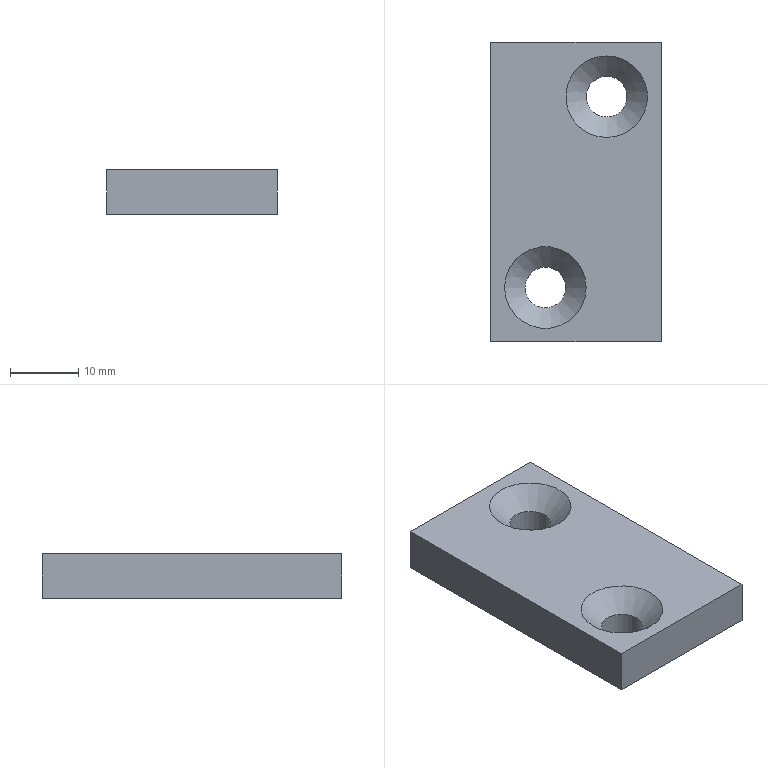Part | NX | features DATUM_CSYS 5, SKETCH 4, DATUM_PLANE 2, SWP104 2, EXTRUDE 1 | 1 solid | 10 faces | box 25 x 44 x 6.5 mm | volume 6556 mm3 | plane 6 | cone 2 | cylinder 2 | commonest cylinder face diameters 6 x2
STEP:
#1=CARTESIAN_POINT('',(12.5,22.,0.));
#2=VERTEX_POINT('',#1);
#3=CARTESIAN_POINT('',(-12.5,22.,0.));
#4=VERTEX_POINT('',#3);
#5=CARTESIAN_POINT('',(12.5,22.,0.));
#6=DIRECTION('',(-1.,0.,0.));
#7=VECTOR('',#6,1000.);
#8=LINE('',#5,#7);
#9=EDGE_CURVE('',#2,#4,#8,.T.);
#10=ORIENTED_EDGE('',*,*,#9,.T.);
#11=CARTESIAN_POINT('',(-12.5,22.,6.5));
#12=VERTEX_POINT('',#11);
#13=CARTESIAN_POINT('',(-12.5,22.,6.5));
#14=DIRECTION('',(0.,0.,-1.));
#15=VECTOR('',#14,1000.);
#16=LINE('',#13,#15);
#17=EDGE_CURVE('',#12,#4,#16,.T.);
#18=ORIENTED_EDGE('',*,*,#17,.F.);
#19=CARTESIAN_POINT('',(12.5,22.,6.5));
#20=VERTEX_POINT('',#19);
#21=CARTESIAN_POINT('',(12.5,22.,6.5));
#22=DIRECTION('',(-1.,0.,0.));
#23=VECTOR('',#22,1000.);
#24=LINE('',#21,#23);
#25=EDGE_CURVE('',#20,#12,#24,.T.);
#26=ORIENTED_EDGE('',*,*,#25,.F.);
#27=CARTESIAN_POINT('',(12.5,22.,6.5));
#28=DIRECTION('',(0.,0.,-1.));
#29=VECTOR('',#28,1000.);
#30=LINE('',#27,#29);
#31=EDGE_CURVE('',#20,#2,#30,.T.);
#32=ORIENTED_EDGE('',*,*,#31,.T.);
#33=EDGE_LOOP('',(#10,#18,#26,#32));
#34=FACE_BOUND('',#33,.T.);
#35=CARTESIAN_POINT('',(12.5,22.,6.5));
#36=DIRECTION('',(0.,-1.,0.));
#37=DIRECTION('',(0.,0.,-1.));
#38=AXIS2_PLACEMENT_3D('',#35,#36,#37);
#39=PLANE('',#38);
#40=ADVANCED_FACE('',(#34),#39,.F.);
#41=CARTESIAN_POINT('',(-12.5,-22.,0.));
#42=VERTEX_POINT('',#41);
#43=CARTESIAN_POINT('',(-12.5,22.,0.));
#44=DIRECTION('',(0.,-1.,0.));
#45=VECTOR('',#44,1000.);
#46=LINE('',#43,#45);
#47=EDGE_CURVE('',#4,#42,#46,.T.);
#48=ORIENTED_EDGE('',*,*,#47,.T.);
#49=CARTESIAN_POINT('',(-12.5,-22.,6.5));
#50=VERTEX_POINT('',#49);
#51=CARTESIAN_POINT('',(-12.5,-22.,6.5));
#52=DIRECTION('',(0.,0.,-1.));
#53=VECTOR('',#52,1000.);
#54=LINE('',#51,#53);
#55=EDGE_CURVE('',#50,#42,#54,.T.);
#56=ORIENTED_EDGE('',*,*,#55,.F.);
#57=CARTESIAN_POINT('',(-12.5,22.,6.5));
#58=DIRECTION('',(0.,-1.,0.));
#59=VECTOR('',#58,1000.);
#60=LINE('',#57,#59);
#61=EDGE_CURVE('',#12,#50,#60,.T.);
#62=ORIENTED_EDGE('',*,*,#61,.F.);
#63=ORIENTED_EDGE('',*,*,#17,.T.);
#64=EDGE_LOOP('',(#48,#56,#62,#63));
#65=FACE_BOUND('',#64,.T.);
#66=CARTESIAN_POINT('',(-12.5,22.,6.5));
#67=DIRECTION('',(1.,0.,0.));
#68=DIRECTION('',(0.,0.,-1.));
#69=AXIS2_PLACEMENT_3D('',#66,#67,#68);
#70=PLANE('',#69);
#71=ADVANCED_FACE('',(#65),#70,.F.);
#72=CARTESIAN_POINT('',(12.5,-22.,0.));
#73=VERTEX_POINT('',#72);
#74=CARTESIAN_POINT('',(-12.5,-22.,0.));
#75=DIRECTION('',(1.,0.,0.));
#76=VECTOR('',#75,1000.);
#77=LINE('',#74,#76);
#78=EDGE_CURVE('',#42,#73,#77,.T.);
#79=ORIENTED_EDGE('',*,*,#78,.T.);
#80=CARTESIAN_POINT('',(12.5,-22.,6.5));
#81=VERTEX_POINT('',#80);
#82=CARTESIAN_POINT('',(12.5,-22.,6.5));
#83=DIRECTION('',(0.,0.,-1.));
#84=VECTOR('',#83,1000.);
#85=LINE('',#82,#84);
#86=EDGE_CURVE('',#81,#73,#85,.T.);
#87=ORIENTED_EDGE('',*,*,#86,.F.);
#88=CARTESIAN_POINT('',(-12.5,-22.,6.5));
#89=DIRECTION('',(1.,0.,0.));
#90=VECTOR('',#89,1000.);
#91=LINE('',#88,#90);
#92=EDGE_CURVE('',#50,#81,#91,.T.);
#93=ORIENTED_EDGE('',*,*,#92,.F.);
#94=ORIENTED_EDGE('',*,*,#55,.T.);
#95=EDGE_LOOP('',(#79,#87,#93,#94));
#96=FACE_BOUND('',#95,.T.);
#97=CARTESIAN_POINT('',(-12.5,-22.,6.5));
#98=DIRECTION('',(0.,1.,0.));
#99=DIRECTION('',(0.,0.,1.));
#100=AXIS2_PLACEMENT_3D('',#97,#98,#99);
#101=PLANE('',#100);
#102=ADVANCED_FACE('',(#96),#101,.F.);
#103=CARTESIAN_POINT('',(12.5,-22.,0.));
#104=DIRECTION('',(0.,1.,0.));
#105=VECTOR('',#104,1000.);
#106=LINE('',#103,#105);
#107=EDGE_CURVE('',#73,#2,#106,.T.);
#108=ORIENTED_EDGE('',*,*,#107,.T.);
#109=ORIENTED_EDGE('',*,*,#31,.F.);
#110=CARTESIAN_POINT('',(12.5,-22.,6.5));
#111=DIRECTION('',(0.,1.,0.));
#112=VECTOR('',#111,1000.);
#113=LINE('',#110,#112);
#114=EDGE_CURVE('',#81,#20,#113,.T.);
#115=ORIENTED_EDGE('',*,*,#114,.F.);
#116=ORIENTED_EDGE('',*,*,#86,.T.);
#117=EDGE_LOOP('',(#108,#109,#115,#116));
#118=FACE_BOUND('',#117,.T.);
#119=CARTESIAN_POINT('',(12.5,-22.,6.5));
#120=DIRECTION('',(-1.,0.,0.));
#121=DIRECTION('',(0.,0.,1.));
#122=AXIS2_PLACEMENT_3D('',#119,#120,#121);
#123=PLANE('',#122);
#124=ADVANCED_FACE('',(#118),#123,.F.);
#125=CARTESIAN_POINT('',(-10.5,-14.043,6.5));
#126=VERTEX_POINT('',#125);
#127=CARTESIAN_POINT('',(-4.5,-14.043,6.5));
#128=DIRECTION('',(0.,0.,-1.));
#129=DIRECTION('',(-1.,0.,0.));
#130=AXIS2_PLACEMENT_3D('',#127,#128,#129);
#131=CIRCLE('',#130,6.);
#132=EDGE_CURVE('',#126,#126,#131,.T.);
#133=ORIENTED_EDGE('',*,*,#132,.T.);
#134=EDGE_LOOP('',(#133));
#135=FACE_BOUND('',#134,.T.);
#136=CARTESIAN_POINT('',(4.5,8.,6.5));
#137=VERTEX_POINT('',#136);
#138=CARTESIAN_POINT('',(4.5,14.,6.5));
#139=DIRECTION('',(0.,0.,1.));
#140=DIRECTION('',(0.,-1.,0.));
#141=AXIS2_PLACEMENT_3D('',#138,#139,#140);
#142=CIRCLE('',#141,6.);
#143=EDGE_CURVE('',#137,#137,#142,.T.);
#144=ORIENTED_EDGE('',*,*,#143,.F.);
#145=EDGE_LOOP('',(#144));
#146=FACE_BOUND('',#145,.T.);
#147=ORIENTED_EDGE('',*,*,#25,.T.);
#148=ORIENTED_EDGE('',*,*,#61,.T.);
#149=ORIENTED_EDGE('',*,*,#92,.T.);
#150=ORIENTED_EDGE('',*,*,#114,.T.);
#151=EDGE_LOOP('',(#147,#148,#149,#150));
#152=FACE_BOUND('',#151,.T.);
#153=CARTESIAN_POINT('',(0.,0.,6.5));
#154=DIRECTION('',(0.,0.,1.));
#155=DIRECTION('',(1.,0.,0.));
#156=AXIS2_PLACEMENT_3D('',#153,#154,#155);
#157=PLANE('',#156);
#158=ADVANCED_FACE('',(#135,#146,#152),#157,.T.);
#159=CARTESIAN_POINT('',(-7.5,-14.043,0.));
#160=VERTEX_POINT('',#159);
#161=CARTESIAN_POINT('',(-4.5,-14.043,0.));
#162=DIRECTION('',(0.,0.,-1.));
#163=DIRECTION('',(-1.,0.,0.));
#164=AXIS2_PLACEMENT_3D('',#161,#162,#163);
#165=CIRCLE('',#164,3.);
#166=EDGE_CURVE('',#160,#160,#165,.T.);
#167=ORIENTED_EDGE('',*,*,#166,.F.);
#168=EDGE_LOOP('',(#167));
#169=FACE_BOUND('',#168,.T.);
#170=CARTESIAN_POINT('',(4.5,11.,0.));
#171=VERTEX_POINT('',#170);
#172=CARTESIAN_POINT('',(4.5,14.,0.));
#173=DIRECTION('',(0.,0.,1.));
#174=DIRECTION('',(0.,-1.,0.));
#175=AXIS2_PLACEMENT_3D('',#172,#173,#174);
#176=CIRCLE('',#175,3.);
#177=EDGE_CURVE('',#171,#171,#176,.T.);
#178=ORIENTED_EDGE('',*,*,#177,.T.);
#179=EDGE_LOOP('',(#178));
#180=FACE_BOUND('',#179,.T.);
#181=ORIENTED_EDGE('',*,*,#9,.F.);
#182=ORIENTED_EDGE('',*,*,#107,.F.);
#183=ORIENTED_EDGE('',*,*,#78,.F.);
#184=ORIENTED_EDGE('',*,*,#47,.F.);
#185=EDGE_LOOP('',(#181,#182,#183,#184));
#186=FACE_BOUND('',#185,.T.);
#187=CARTESIAN_POINT('',(0.,0.,0.));
#188=DIRECTION('',(0.,0.,1.));
#189=DIRECTION('',(1.,0.,0.));
#190=AXIS2_PLACEMENT_3D('',#187,#188,#189);
#191=PLANE('',#190);
#192=ADVANCED_FACE('',(#169,#180,#186),#191,.F.);
#193=CARTESIAN_POINT('',(4.5,11.,3.5));
#194=VERTEX_POINT('',#193);
#195=CARTESIAN_POINT('',(4.5,14.,3.5));
#196=DIRECTION('',(0.,0.,1.));
#197=DIRECTION('',(0.,-1.,0.));
#198=AXIS2_PLACEMENT_3D('',#195,#196,#197);
#199=CIRCLE('',#198,3.);
#200=EDGE_CURVE('',#194,#194,#199,.F.);
#201=ORIENTED_EDGE('',*,*,#200,.T.);
#202=EDGE_LOOP('',(#201));
#203=FACE_BOUND('',#202,.T.);
#204=ORIENTED_EDGE('',*,*,#143,.T.);
#205=EDGE_LOOP('',(#204));
#206=FACE_BOUND('',#205,.T.);
#207=CARTESIAN_POINT('',(4.5,14.,6.5));
#208=DIRECTION('',(0.,0.,1.));
#209=DIRECTION('',(0.,-1.,0.));
#210=AXIS2_PLACEMENT_3D('',#207,#208,#209);
#211=CONICAL_SURFACE('',#210,6.,0.7854);
#212=ADVANCED_FACE('',(#203,#206),#211,.F.);
#213=ORIENTED_EDGE('',*,*,#177,.F.);
#214=EDGE_LOOP('',(#213));
#215=FACE_BOUND('',#214,.T.);
#216=ORIENTED_EDGE('',*,*,#200,.F.);
#217=EDGE_LOOP('',(#216));
#218=FACE_BOUND('',#217,.T.);
#219=CARTESIAN_POINT('',(4.5,14.,6.5));
#220=DIRECTION('',(0.,0.,1.));
#221=DIRECTION('',(0.,-1.,0.));
#222=AXIS2_PLACEMENT_3D('',#219,#220,#221);
#223=CYLINDRICAL_SURFACE('',#222,3.);
#224=ADVANCED_FACE('',(#215,#218),#223,.F.);
#225=CARTESIAN_POINT('',(-7.5,-14.043,3.5));
#226=VERTEX_POINT('',#225);
#227=CARTESIAN_POINT('',(-4.5,-14.043,3.5));
#228=DIRECTION('',(0.,0.,-1.));
#229=DIRECTION('',(-1.,0.,0.));
#230=AXIS2_PLACEMENT_3D('',#227,#228,#229);
#231=CIRCLE('',#230,3.);
#232=EDGE_CURVE('',#226,#226,#231,.F.);
#233=ORIENTED_EDGE('',*,*,#232,.F.);
#234=EDGE_LOOP('',(#233));
#235=FACE_BOUND('',#234,.T.);
#236=ORIENTED_EDGE('',*,*,#132,.F.);
#237=EDGE_LOOP('',(#236));
#238=FACE_BOUND('',#237,.T.);
#239=CARTESIAN_POINT('',(-4.5,-14.043,6.5));
#240=DIRECTION('',(0.,0.,1.));
#241=DIRECTION('',(1.,0.,0.));
#242=AXIS2_PLACEMENT_3D('',#239,#240,#241);
#243=CONICAL_SURFACE('',#242,6.,0.7854);
#244=ADVANCED_FACE('',(#235,#238),#243,.F.);
#245=ORIENTED_EDGE('',*,*,#166,.T.);
#246=EDGE_LOOP('',(#245));
#247=FACE_BOUND('',#246,.T.);
#248=ORIENTED_EDGE('',*,*,#232,.T.);
#249=EDGE_LOOP('',(#248));
#250=FACE_BOUND('',#249,.T.);
#251=CARTESIAN_POINT('',(-4.5,-14.043,-4.1));
#252=DIRECTION('',(0.,0.,-1.));
#253=DIRECTION('',(-1.,0.,0.));
#254=AXIS2_PLACEMENT_3D('',#251,#252,#253);
#255=CYLINDRICAL_SURFACE('',#254,3.);
#256=ADVANCED_FACE('',(#247,#250),#255,.F.);
#257=CLOSED_SHELL('',(#40,#71,#102,#124,#158,#192,#212,#224,#244,#256));
#258=MANIFOLD_SOLID_BREP('',#257);
#259=(LENGTH_UNIT()NAMED_UNIT(*)SI_UNIT(.MILLI.,.METRE.));
#260=UNCERTAINTY_MEASURE_WITH_UNIT(LENGTH_MEASURE(0.00001),#259,'','');
#261=(NAMED_UNIT(*)PLANE_ANGLE_UNIT()SI_UNIT($,.RADIAN.));
#262=(NAMED_UNIT(*)SI_UNIT($,.STERADIAN.)SOLID_ANGLE_UNIT());
#263=(GEOMETRIC_REPRESENTATION_CONTEXT(3)GLOBAL_UNCERTAINTY_ASSIGNED_CONTEXT((#260))GLOBAL_UNIT_ASSIGNED_CONTEXT((#259,#261,#262))REPRESENTATION_CONTEXT('',''));
#264=ADVANCED_BREP_SHAPE_REPRESENTATION('',(#258),#263);